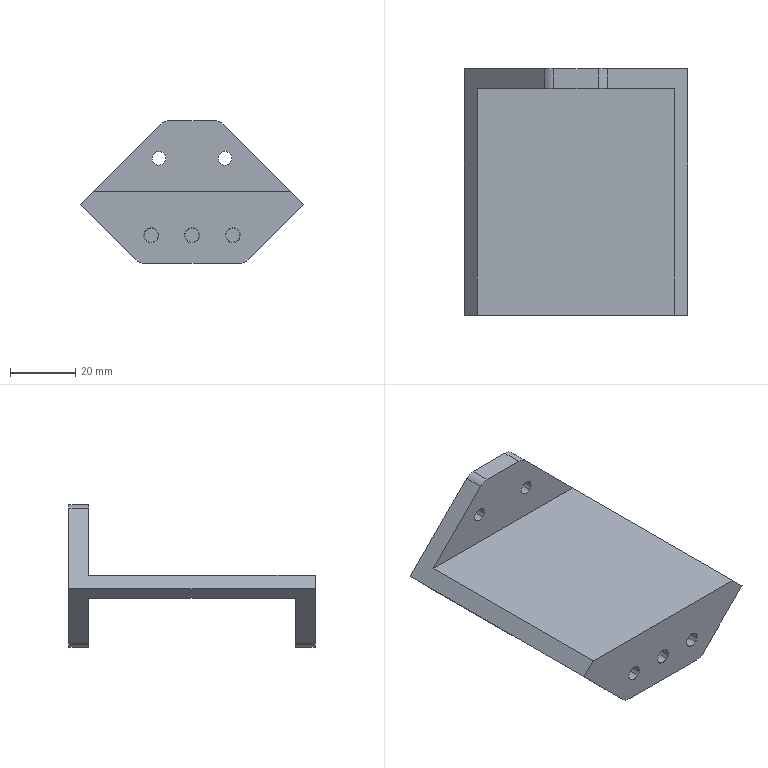NC program | NX | posted with a generic post | part box 68.307 x 75.3 x 43.668 mm
Lines 19 to 906 of 9000:
(ADAPTIVE_MILLING , TOOL : D10)
N36 T15 M6
N38 G54
N40 G17 G0 G90 X-31.665 Y-45.86 B0. C0. S9500 M3
N42 G43 Z30. H15
N44 Z-11.85
N46 G94 G1 Z-14.85 F1000.
N48 X-31.386 Y-45.079 F3000.
N50 X-31.129 Y-44.291
N52 G3 X-31.665 Y-43.213 R1.017
N54 X-34.729 Y-42.452 R8.28
N56 X-39.219 Y-42.188 R149.722
N58 G2 X-43.375 Y-39.245 R6.16
N60 X-45.215 Y-33.584 R13.81
N62 X-45.618 Y-24.224 R80.865
N64 G1 X-45.625 Y-22.724
N66 X-45.631 Y-20.599
N68 X-45.634 Y-17.349
N70 X-45.636 Y-9.599
N72 Y35.151
N74 X-45.629 Y35.401
N76 G2 X-43.02 Y39.625 R5.889
N78 X-37.31 Y41.673 R12.902
N80 X-28.577 Y42.113 R68.398
N82 G1 X-27.202 Y42.123
N84 X-25.702 Y42.13
N86 X-23.577 Y42.135
N88 X-19.952 Y42.138
N90 X-9.327 Y42.139
N92 X38.673
N94 G2 X42.915 Y39.817 R5.625
N96 X45.077 Y34.419 R11.908
N98 X45.604 Y25.819 R57.608
N100 G1 X45.614 Y24.694
N102 X45.621 Y23.444
N104 X45.628 Y21.694
N106 X45.633 Y19.319
N108 X45.635 Y14.944
N110 X45.636 Y-13.681
N112 Y-35.181
N114 X45.634 Y-35.306
N116 X45.627 Y-35.431
N118 X45.617 Y-35.555
N120 G2 X42.912 Y-39.721 R5.935
N122 X37.297 Y-41.68 R13.094
N124 X28.689 Y-42.113 R69.339
N126 G1 X27.439 Y-42.122
N128 X25.939 Y-42.129
N130 X23.814 Y-42.134
N132 X20.439 Y-42.138
N134 X11.689 Y-42.139
N136 X-27.811
N138 G2 X-33.408 Y-41.614 R60.129
N140 X-37.011 Y-41.244 R40.3
N142 X-42.457 Y-36.811 R8.328
N144 X-44.258 Y-30.091 R18.441
N146 X-44.608 Y-19.851 R114.492
N148 G1 X-44.615 Y-18.101
N150 X-44.621 Y-15.601
N152 X-44.624 Y-11.601
N154 X-44.625 Y-0.101
N156 Y32.149
N158 X-44.618 Y32.399
N160 G2 X-40.842 Y38.536 R7.705
N162 X-34.357 Y40.647 R15.817
N164 X-24.623 Y41.102 R84.301
N166 G1 X-23.373 Y41.111
N168 X-21.873 Y41.117
N170 X-19.623 Y41.123
N172 X-16.123 Y41.127
N174 X-7.873 Y41.128
N176 X35.502
N178 G2 X41.889 Y37.582 R7.573
N180 X44.088 Y31.26 R15.12
N182 X44.589 Y22.281 R70.625
N184 G1 X44.599 Y21.156
N186 X44.608 Y19.781
N188 X44.615 Y18.156
N190 X44.621 Y15.781
N192 X44.624 Y12.031
N194 X44.625 Y2.156
N196 Y-32.094
N198 X44.624 Y-32.219
N200 X44.615 Y-32.469
N202 X44.609 Y-32.594
N204 X44.6 Y-32.718
N206 G2 X40.792 Y-38.576 R7.743
N208 X34.544 Y-40.625 R15.694
N210 X25.187 Y-41.098 R77.266
N212 G1 X23.937 Y-41.108
N214 X22.312 Y-41.116
N216 X20.312 Y-41.122
N218 X17.187 Y-41.126
N220 X11.187 Y-41.128
N222 X-25.438
N224 G2 X-34.656 Y-40.436 R83.781
N226 X-41.245 Y-35.347 R9.432
N228 G1 X-41.361 Y-35.125
N230 X-41.417 Y-35.013
N232 X-41.472 Y-34.901
N234 X-41.525 Y-34.788
N236 X-41.578 Y-34.675
N238 X-41.63 Y-34.561
N240 X-41.73 Y-34.332
N242 X-41.779 Y-34.217
N244 X-41.827 Y-34.101
N246 X-41.873 Y-33.985
N248 X-41.923 Y-33.871
N250 X-41.974 Y-33.78
N252 G2 X-42.882 Y-31.037 R6.648
N254 X-43.558 Y-21.32 R65.424
N256 G1 X-43.571 Y-20.445
N258 X-43.583 Y-19.321
N260 X-43.592 Y-18.071
N262 X-43.6 Y-16.446
N264 X-43.607 Y-14.321
N266 X-43.611 Y-11.321
N268 X-43.614 Y-5.946
N270 X-43.615 Y29.304
N272 X-43.613 Y29.554
N274 X-43.612 Y29.679
N276 X-43.609 Y29.804
N278 X-43.601 Y30.054
N280 X-43.595 Y30.179
N282 G2 X-38.917 Y37.549 R8.918
N284 X-31.774 Y39.66 R18.511
N286 X-20.663 Y40.098 R106.491
N288 G1 X-18.913 Y40.106
N290 X-16.663 Y40.111
N292 X-13.288 Y40.115
N294 X-6.288 Y40.117
N296 X32.962 Y40.118
N298 X33.212 Y40.115
N300 G2 X41.065 Y35.398 R8.902
N302 G1 X41.128 Y35.29
N304 X41.189 Y35.181
N306 X41.307 Y34.96
N308 X41.364 Y34.849
N310 X41.42 Y34.738
N312 X41.53 Y34.513
N314 X41.583 Y34.4
N316 X41.688 Y34.173
N318 X41.723 Y34.111
N320 G2 X42.741 Y31.774 R5.072
N322 X43.532 Y22.569 R54.427
N324 X43.614 Y1.695 R975.422
N326 G1 X43.615 Y-29.43
N328 X43.612 Y-29.68
N330 X43.606 Y-29.93
N332 X43.602 Y-30.055
N334 X43.589 Y-30.305
N336 G2 X38.924 Y-37.552 R8.898
N338 X32.277 Y-39.599 R17.939
N340 X21.795 Y-40.089 R90.439
N342 G1 X20.42 Y-40.099
N344 X18.67 Y-40.106
N346 X16.295 Y-40.112
N348 X12.67 Y-40.116
N350 X4.42 Y-40.117
N352 X-23.705 Y-40.118
N354 G2 X-32.804 Y-39.541 R64.009
N356 X-38.655 Y-36.183 R10.283
N358 G3 X-40.291 Y-35.45 R29.243
N360 G2 X-42.026 Y-33.711 R5.781
N362 G1 X-42.148 Y-33.521
N364 X-42.605 Y-32.397
N366 X-42.64 Y-32.264
N368 X-42.796 Y-31.024
N370 X-42.8 Y-30.958
N372 Y30.958
N374 X-42.796 Y31.024
N376 G2 X-41.347 Y34.608 R5.58
N378 X-37.507 Y36.891 R13.071
N380 X-28.873 Y38.771 R27.669
N382 X-15.38 Y39.097 R191.104
N384 G1 X-12.505 Y39.103
N386 X-8.005 Y39.106
N388 X6.37 Y39.107
N390 X30.62
N392 X30.995 Y39.103
N394 X31.245 Y39.098
N396 G2 X38.235 Y36.245 R9.765
N398 G3 X39.054 Y35.991 R2.422
N400 G2 X41.347 Y34.608 R5.838
N402 G1 X41.724 Y34.11
N404 G3 X43.518 Y34.789 R1.001
N406 G1 X43.448 Y35.087 Z-14.835
N408 X43.331 Y35.371 Z-14.819
N410 X42.801 Y36.651 Z-14.75
N412 X42.476 Y37.441
N414 X42.137 Y38.226
N416 G3 X41.724 Y38.61 R1.054
N418 G1 X37.807 Y40.557
N420 G3 X34.63 Y41.648 R15.261
N422 X32.101 Y41.977 R26.338
N424 G1 X30.702 Y42.068
N426 X29.301 Y42.103
N428 X-18.201 Y42.154
N430 G3 X-28.49 Y41.809 R149.233
N432 X-35.16 Y40.765 R46.348
N434 G1 X-39.008 Y39.867
N436 G3 X-39.589 Y39.481 R1.032
N438 G1 X-40.629 Y38.048
N440 X-41.045 Y37.481 Z-14.785
N442 X-41.447 Y36.904 Z-14.82
N444 G3 X-41.554 Y36.33 Z-14.85 R1.049
N446 X-40.172 Y35.52 R1.003
N448 G2 X-37.932 Y36.172 R5.778
N450 X-28.564 Y37.701 R71.762
N452 X-13.947 Y38.085 R197.198
N454 G1 X-11.697 Y38.09
N456 X-7.947 Y38.094
N458 X-0.322 Y38.096
N460 X28.553
N462 X28.927 Y38.092
N464 X29.427 Y38.082
N466 G2 X35.518 Y36.429 R13.144
N468 G3 X36.153 Y36.203 R3.775
N470 G2 X38.677 Y36.061 R11.846
N472 G3 X38.828 Y38.251 R-1.1
N474 G1 X31.219 Y38.258
N476 X29.219 Y38.26 Z-14.75
N478 X-29.334 Y38.312
N480 X-31.334 Y38.314 Z-14.85
N482 X-38.327 Y38.32
N484 G3 X-38.178 Y36.13 R-1.1
N486 G1 X-37.686 Y36.198
N488 X-37.614 Y36.203
N490 G3 X-30.501 Y36.53 R56.138
N492 G2 X-13.515 Y37.07 R208.339
N494 G1 X-11.14 Y37.077
N496 X-7.89 Y37.081
N498 X-2.39 Y37.084
N500 X19.11 Y37.085
N502 X26.485
N504 X26.985 Y37.083
N506 G2 X32.731 Y36.203 R19.314
N508 G1 X36.231
N510 G3 X37.329 Y37.305 R1.1
N512 X36.231 Y38.403 R1.1
N514 G1 X31.619
N516 X29.619 Z-14.75
N518 X-29.592
N520 X-31.592 Z-14.85
N522 X-34.989
N524 G3 X-36.087 Y37.301 R1.1
N526 X-34.989 Y36.203 R1.1
N528 G1 X-31.686
N530 X-31.614 Y36.198
N532 G3 X-25.758 Y35.917 R31.279
N534 G2 X-1.884 Y36.073 R956.691
N536 G1 X12.116 Y36.075
N538 X24.616
N540 X25.366 Y36.07
N542 X25.741 Y36.063
N544 X25.991 Y36.057
N546 G2 X29.473 Y35.738 R41.584
N548 G3 X30.379 Y36.028 R4.567
N550 G2 X32.811 Y36.203 R10.972
N552 G3 X33.909 Y37.305 R1.1
N554 X32.808 Y38.403 R1.1
N556 G1 X31.571 Y38.399
N558 X29.571 Y38.392 Z-14.75
N560 X-29.041 Y38.192
N562 X-30.249 Y38.177 Z-14.81
N564 G3 X-30.926 Y37.801 Z-14.85 R1.132
N566 X-30.379 Y36.028 R1.102
N568 X-25.86 Y35.125 R12.1
N570 X-13.112 Y35.059 R322.419
N572 G1 X-12.237 Y35.061
N574 X-11.737 Y35.063
N576 X-10.487
N578 X-9.737 Y35.066
N580 X-8.737
N582 X-8.362
N584 X-7.362 Y35.069
N586 X-6.612
N588 X-5.612 Y35.071
N590 X-5.112 Y35.072
N592 X-4.362 Y35.071
N594 X-3.237 Y35.073
N596 X-2.862 Y35.074
N598 X-1.987 Y35.073
N600 X-0.737 Y35.075
N602 X0.513 Y35.072
N604 X1.138 Y35.074
N606 X2.638 Y35.073
N608 X3.513 Y35.071
N610 X4.138 Y35.073
N612 X5.513 Y35.072
N614 X6.138
N616 X7.263 Y35.075
N618 X8.263 Y35.073
N620 X9.513 Y35.076
N622 X10.138 Y35.075
N624 X11.638 Y35.076
N626 X12.138 Y35.077
N628 X13.138 Y35.074
N630 X14.513 Y35.077
N632 X15.638 Y35.074
N634 X16.388 Y35.075
N636 X17.263 Y35.074
N638 X17.763 Y35.073
N640 X18.638 Y35.075
N642 X19.888 Y35.073
N644 G2 X27.883 Y34.883 R129.556
N646 G3 X29.009 Y35.451 R1.838
N648 G1 X29.128 Y35.52
N650 X29.819 Y35.811
N652 G3 X30.291 Y37.458 R1.103
N654 X29.296 Y37.925 Z-14.793 R1.131
N656 G1 X28.445 Y37.924 Z-14.75
N658 X-28.234 Y37.863
N660 X-28.821 Y37.865 Z-14.779
N662 X-29.408 Y37.85 Z-14.809
N664 G3 X-30.105 Y37.445 Z-14.85 R1.13
N666 X-29.67 Y35.749 R1.103
N668 G2 X-28.24 Y35.038 R22.99
N670 G3 X-23.33 Y34.207 R16.333
N672 X-8.332 Y34.071 R360.005
N674 G1 X-7.832 Y34.072
N676 X-6.832 Y34.071
N678 X-5.707 Y34.073
N680 X-4.707 Y34.072
N682 X-3.707 Y34.074
N684 X-3.082
N686 X-2.332 Y34.073
N688 X-0.957 Y34.075
N690 X0.418 Y34.072
N692 X1.793 Y34.075
N694 X2.418 Y34.073
N696 X3.918 Y34.074
N698 X4.918 Y34.076
N700 X5.793 Y34.074
N702 X6.543 Y34.075
N704 X6.918 Y34.076
N706 X8.293 Y34.073
N708 G2 X23.793 Y34.017 R790.06
N710 G3 X27.283 Y34.08 R15.903
N712 X28.051 Y34.706 R1.755
N714 G1 X28.544 Y35.09
N716 G3 X28.832 Y36.49 R1.106
N718 X27.784 Y37.059 Z-14.787 R1.123
N720 G1 X27.042 Y37.064 Z-14.75
N722 X-27.468 Y37.414
N724 X-28.489 Y37.408 Z-14.801
N726 G3 X-29.277 Y36.885 Z-14.85 R1.117
N728 X-29.009 Y35.451 R1.106
N730 X-25.203 Y33.695 R7.328
N732 X-17.983 Y33.139 R44.306
N734 G1 X-17.108 Y33.125
N736 X-15.983 Y33.111
N738 X-14.733 Y33.1
N740 X-13.483 Y33.093
N742 X-12.733 Y33.09
N744 X-11.983 Y33.084
N746 X-11.108 Y33.081
N748 X17.392 Y33.082
N750 X17.892 Y33.079
N752 X20.391 Y33.061
N754 G3 X25.639 Y33.067 R60.63
N756 X27.062 Y33.478 R2.885
N758 G1 X27.155 Y33.562
N760 X27.221 Y33.641
N762 X27.825 Y34.438
N764 G3 X27.878 Y35.689 R1.108
N766 X26.78 Y36.204 Z-14.786 R1.183
N768 G1 X26.057 Y36.212 Z-14.75
N770 X-26.656 Y36.796
N772 X-27.692 Z-14.802
N774 G3 X-28.476 Y36.29 Z-14.85 R1.117
N776 X-28.219 Y34.837 R1.106
N778 X-27.214 Y33.943 R12.106
N780 X-22.949 Y32.611 R11.114
N782 X-14.343 Y32.133 R70.206
N784 G1 X-13.343 Y32.12
N786 X-12.343 Y32.111
N788 X-11.093 Y32.104
N790 X-9.218 Y32.098
N792 X-6.343 Y32.094
N794 X-0.593 Y32.092
N796 X14.407
N798 X14.907 Y32.09
N800 G3 X24.031 Y32.072 R239.487
N802 X26.574 Y32.634 R6.287
N804 X27.152 Y33.521 R1.675
N806 G1 X27.221 Y33.641
N808 X27.296 Y33.741
N810 G3 X27.352 Y34.989 R1.108
N812 X26.255 Y35.507 Z-14.786 R1.183
N814 G1 X25.532 Y35.518 Z-14.75
N816 X-26.08 Y36.26
N818 X-26.624 Y36.271 Z-14.777
N820 X-27.167 Y36.26 Z-14.804
N822 G3 X-27.915 Y35.785 Z-14.85 R1.127
N824 X-27.878 Y34.508 R1.108
N826 X-25. Y32.426 R5.204
N828 X-18.61 Y31.349 R24.488
N830 X-4.614 Y31.107 R256.473
N832 G1 X-0.489 Y31.104
N834 X11.386 Y31.103
N836 X11.886 Y31.1
N838 G3 X22.635 Y31.084 R342.387
N840 X26.16 Y31.801 R8.623
N842 X26.695 Y32.397 R1.269
N844 G1 X26.978 Y33.092
N846 G3 X26.808 Y34.206 R1.112
N848 X25.79 Y34.61 Z-14.793 R1.215
N850 G1 X24.93 Y34.628 Z-14.75
N852 X-25.608 Y35.656
N854 X-26.157 Y35.671 Z-14.777
N856 X-26.706 Y35.664 Z-14.805
N858 G3 X-27.452 Y35.203 Z-14.85 R1.127
N860 X-27.425 Y33.911 R1.108
N862 X-24.67 Y31.711 R5.118
N864 X-18.317 Y30.449 R22.393
N866 X-4.824 Y30.123 R190.213
N868 G1 X-2.074 Y30.118
N870 X2.301 Y30.115
N872 X8.426 Y30.114
N874 X8.926 Y30.111
N876 X10.426 Y30.101
N878 X11.051 Y30.1
N880 X12.176 Y30.093
N882 G3 X22.049 Y30.129 R195.88
N884 X25.694 Y30.906 R9.913
N886 X26.66 Y32.264 R1.466
N888 G1 X26.691 Y32.385
N890 G3 X26.467 Y33.373 R1.116
N892 X25.46 Y33.767 Z-14.794 R1.223
N894 G1 X24.583 Y33.789 Z-14.75
N896 X-25.125 Y35.011
N898 X-25.7 Y35.028 Z-14.779
N900 X-26.276 Y35.027 Z-14.808
N902 G3 X-26.996 Y34.618 Z-14.85 R1.129
N904 X-27.152 Y33.521 R1.112
N906 X-25.276 Y31.434 R3.812
N908 X-19.931 Y29.788 R15.223
N910 X-9.831 Y29.184 R79.227
N912 G1 X-8.831 Y29.171
N914 X-7.581 Y29.158
N916 X-6.081 Y29.148
N918 X-4.331 Y29.139
N920 X-2.081 Y29.133
N922 X1.044 Y29.128
N924 X5.544 Y29.125
N926 X7.419 Y29.112
N928 X8.169 Y29.111
N930 X9.294 Y29.105
N932 X10.418 Y29.097
N934 X11.418 Y29.095
N936 G3 X21.291 Y29.164 R170.676
N938 X25.528 Y30.126 R10.894
N940 X26.524 Y31.183 R1.743
N942 G1 X26.618 Y31.927
N944 G3 X26.277 Y32.867 R1.116
N946 X25.371 Y33.169 Z-14.801 R1.236
N948 G1 X24.354 Y33.196 Z-14.75
N950 X-24.875 Y34.544
N952 X-25.475 Y34.562 Z-14.78
N954 X-26.075 Y34.565 Z-14.81
N956 G3 X-26.768 Y34.203 Z-14.85 R1.132
N958 X-26.964 Y33.058 R1.111
N960 X-24.796 Y30.583 R4.334
N962 X-19.092 Y28.832 R16.394
N964 X-8.994 Y28.207 R80.514
N966 G1 X-7.994 Y28.192
N968 X-6.869 Y28.178
N970 X-5.494 Y28.166
N972 X-3.869 Y28.156
N974 X-1.994 Y28.148
N976 X0.631 Y28.142
N978 X2.506 Y28.139
N980 X3.506 Y28.132
N982 X4.256 Y28.13
N984 X5.381 Y28.122
N986 X6.381 Y28.12
N988 X7.631 Y28.111
N990 X8.631 Y28.108
N992 X9.256 Y28.104
N994 X10.006 Y28.098
N996 X10.756 Y28.096
N998 G3 X20.504 Y28.191 R154.869
N1000 X25.23 Y29.251 R12.567
N1002 X26.425 Y30.304 R2.404
N1004 X26.535 Y31.272 R5.757
N1006 X26.133 Y32.266 R1.112
N1008 X25.278 Y32.514 Z-14.805 R1.281
N1010 G1 X24.189 Y32.546 Z-14.75
N1012 X-24.629 Y33.963
N1014 X-25.836 Y33.987 Z-14.81
N1016 G3 X-26.526 Y33.631 Z-14.85 R1.132
N1018 X-26.728 Y32.479 R1.111
N1020 X-25.119 Y30.213 R3.683
N1022 X-19.924 Y28.163 R13.518
N1024 X-10.852 Y27.296 R54.918
N1026 X10.647 Y27.095 R999.171
N1028 X20.018 Y27.235 R135.2
N1030 X25.095 Y28.432 R13.579
N1032 X26.402 Y29.556 R3.006
N1034 X26.5 Y30.673 R2.968
N1036 X26.051 Y31.56 R1.116
N1038 X25.246 Y31.779 Z-14.808 R1.29
N1040 G1 X24.097 Y31.818 Z-14.75
N1042 X-24.421 Y33.462
N1044 X-25.064 Y33.489 Z-14.782
N1046 X-25.709 Y33.492 Z-14.815
N1048 G3 X-26.337 Y33.187 Z-14.85 R1.143
N1050 X-26.66 Y32.264 R1.116
N1052 X-25.246 Y29.724 R3.468
N1054 X-20.29 Y27.446 R12.353
N1056 X-11.369 Y26.373 R45.968
N1058 X11.253 Y26.107 R715.221
N1060 X20.245 Y26.349 R87.619
N1062 X25.152 Y27.703 R12.778
N1064 X26.419 Y28.871 R2.969
N1066 X26.5 Y29.952 R3.319
N1068 X25.986 Y30.883 R1.113
N1070 X25.252 Y31.059 Z-14.812 R1.327
N1072 G1 X24.019 Y31.106 Z-14.75
N1074 X-24.253 Y32.957
N1076 X-24.937 Y32.986 Z-14.784
N1078 X-25.621 Y32.999 Z-14.819
N1080 G3 X-26.196 Y32.761 Z-14.85 R1.153
N1082 X-26.598 Y31.768 R1.112
N1084 X-25.111 Y28.992 R3.753
N1086 X-19.955 Y26.559 R12.83
N1088 X-10.918 Y25.414 R45.657
N1090 X16.578 Y25.166 R596.971
N1092 X23.245 Y26.086 R25.616
N1094 X26.24 Y27.815 R6.59
N1096 X26.5 Y28.443 R1.55
N1098 G1 Y29.318
N1100 G3 X25.979 Y30.254 R1.113
N1102 X25.252 Y30.425 Z-14.812 R1.335
N1104 G1 X24.01 Y30.473 Z-14.75
N1106 X-24.152 Y32.336
N1108 X-25.539 Y32.379 Z-14.819
N1110 G3 X-26.1 Y32.155 Z-14.85 R1.156
N1112 X-26.52 Y31.147 R1.112
N1114 X-25.327 Y28.555 R3.487
N1116 X-20.433 Y25.893 R11.764
N1118 X-11.685 Y24.523 R38.906
N1120 X6.559 Y24.132 R367.265
N1122 X17.806 Y24.286 R168.743
N1124 X24.025 Y25.553 R19.875
N1126 X26.345 Y27.19 R5.403
N1128 G1 X26.5 Y27.668
N1130 Y28.543
N1132 G3 X25.978 Y29.479 R1.113
N1134 X25.255 Y29.65 Z-14.812 R1.339
N1136 G1 X24.01 Y29.703 Z-14.75
N1138 X-24.071 Y31.752
N1140 X-24.801 Y31.789 Z-14.787
N1142 X-25.532 Y31.8 Z-14.823
N1144 X-25.791 Y31.732 Z-14.837
N1146 X-26.029 Y31.61 Z-14.85
N1148 G3 X-26.5 Y30.708 R1.116
N1150 X-25.43 Y28.003 R3.502
N1152 X-20.761 Y25.202 R11.243
N1154 X-12.051 Y23.624 R35.558
N1156 X3.065 Y23.174 R247.766
N1158 X16.562 Y23.269 R235.069
N1160 X23.43 Y24.483 R23.969
N1162 X26.256 Y26.262 R6.78
N1164 X26.5 Y26.867 R1.695
N1166 G1 Y27.742
N1168 G3 X25.978 Y28.678 R1.112
N1170 X25.261 Y28.85 Z-14.813 R1.345
N1172 G1 X24.01 Y28.911 Z-14.75
N1174 X-24.009 Y31.241
N1176 X-24.76 Y31.282 Z-14.788
N1178 X-25.512 Y31.302 Z-14.825
N1180 X-25.752 Y31.246 Z-14.838
N1182 X-25.977 Y31.144 Z-14.85
N1184 G3 X-26.5 Y30.208 R1.112
N1186 X-25.385 Y27.262 R3.757
N1188 X-20.635 Y24.354 R11.638
N1190 X-11.567 Y22.664 R36.07
N1192 X5.173 Y22.173 R256.984
N1194 X16.669 Y22.335 R158.056
N1196 X23.628 Y23.723 R23.026
N1198 X26.299 Y25.512 R6.447
N1200 X26.5 Y26.068 R2.148
N1202 G1 Y26.943
N1204 G3 X25.978 Y27.879 R1.112
N1206 X25.264 Y28.052 Z-14.813 R1.349
N1208 G1 X24.01 Y28.117 Z-14.75
N1210 X-23.994 Y30.611
N1212 X-24.749 Y30.654 Z-14.788
N1214 X-25.505 Y30.678 Z-14.826
N1216 X-25.742 Y30.624 Z-14.838
N1218 X-25.964 Y30.527 Z-14.85
N1220 G3 X-26.5 Y29.583 R1.112
N1222 X-25.273 Y26.425 R3.967
N1224 X-20.291 Y23.419 R12.343
N1226 X-10.975 Y21.691 R37.38
N1228 X5.889 Y21.184 R248.054
N1230 X17.255 Y21.454 R113.525
N1232 X24.036 Y23.055 R21.152
N1234 X26.329 Y24.741 R5.988
N1236 X26.5 Y25.244 R4.161
N1238 G1 Y26.119
N1240 G3 X25.977 Y27.055 R1.112
N1242 X25.268 Y27.228 Z-14.813 R1.367
N1244 G1 X24.01 Y27.298 Z-14.75
N1246 X-23.994 Y29.981
N1248 X-24.747 Y30.027 Z-14.788
N1250 X-25.502 Y30.053 Z-14.826
N1252 X-25.74 Y30. Z-14.838
N1254 X-25.964 Y29.902 Z-14.85
N1256 G3 X-26.5 Y28.958 R1.112
N1258 X-25.256 Y25.676 R4.111
N1260 X-20.311 Y22.607 R12.506
N1262 X-11.392 Y20.802 R35.936
N1264 X3.968 Y20.219 R197.271
N1266 X15.838 Y20.397 R147.671
N1268 X23.405 Y21.927 R25.574
N1270 X26.286 Y23.85 R7.054
N1272 X26.5 Y24.429 R1.888
N1274 G1 Y25.304
N1276 G3 X25.977 Y26.241 R1.112
N1278 X25.269 Y26.414 Z-14.813 R1.369
N1280 G1 X24.01 Y26.486 Z-14.75
N1282 X-23.994 Y29.229
N1284 X-24.747 Y29.276 Z-14.788
N1286 X-25.501 Y29.303 Z-14.826
N1288 X-25.74 Y29.25 Z-14.838
N1290 X-25.964 Y29.152 Z-14.85
N1292 G3 X-26.5 Y28.208 R1.112
N1294 X-25.252 Y24.923 R4.193
N1296 X-20.226 Y21.751 R12.717
N1298 X-11.322 Y19.874 R35.586
N1300 X4.16 Y19.237 R182.936
N1302 X16.152 Y19.488 R120.826
N1304 X23.45 Y21.087 R24.765
N1306 X26.308 Y23.042 R6.971
N1308 X26.5 Y23.581 R2.45
N1310 G1 Y24.456
N1312 G3 X25.977 Y25.393 R1.112
N1314 X25.271 Y25.566 Z-14.813 R1.372
N1316 G1 X24.01 Y25.64 Z-14.75
N1318 X-23.994 Y28.476
N1320 X-24.746 Y28.525 Z-14.788
N1322 X-25.499 Y28.553 Z-14.825
N1324 X-25.739 Y28.5 Z-14.838
N1326 X-25.964 Y28.402 Z-14.85
N1328 G3 X-26.5 Y27.458 R1.112
N1330 X-25.258 Y24.168 R4.254
N1332 X-20.153 Y20.889 R12.966
N1334 X-10.89 Y18.906 R36.206
N1336 X5.466 Y18.243 R188.956
N1338 X17.199 Y18.673 R89.943
N1340 X24.164 Y20.557 R21.586
N1342 X26.386 Y22.329 R5.518
N1344 X26.5 Y23.605 R3.126
N1346 X25.977 Y24.541 R1.112
N1348 X25.275 Y24.715 Z-14.813 R1.377
N1350 G1 X24.01 Y24.795 Z-14.75
N1352 X-23.994 Y27.845
N1354 X-24.744 Y27.898 Z-14.788
N1356 X-25.495 Y27.928 Z-14.825
N1358 X-25.737 Y27.876 Z-14.838
N1360 X-25.963 Y27.777 Z-14.85
N1362 G3 X-26.5 Y26.833 R1.112
N1364 X-25.271 Y23.41 R4.371
N1366 X-20.203 Y20.072 R13.063
N1368 X-10.715 Y17.962 R36.054
N1370 X4.639 Y17.272 R172.068
N1372 X16.499 Y17.663 R95.948
N1374 X23.742 Y19.484 R23.837
N1376 X26.337 Y21.386 R6.695
N1378 X26.5 Y21.875 R6.215
N1380 G1 Y22.75
N1382 G3 X25.977 Y23.687 R1.112
N1384 X25.277 Y23.86 Z-14.814 R1.38
N1386 G1 X24.01 Y23.943 Z-14.75
N1388 X-23.994 Y27.093
N1390 X-24.743 Y27.146 Z-14.788
N1392 X-25.494 Y27.179 Z-14.825
N1394 X-25.736 Y27.126 Z-14.838
N1396 X-25.963 Y27.028 Z-14.85
N1398 G3 X-26.5 Y26.083 R1.112
N1400 X-25.21 Y22.555 R4.477
N1402 X-20.03 Y19.159 R13.513
N1404 X-10.548 Y17.018 R36.446
N1406 X5.554 Y16.283 R170.558
N1408 X17.156 Y16.822 R81.323
N1410 X24.209 Y18.85 R21.831
N1412 X26.345 Y20.543 R6.042
N1414 G1 X26.5 Y21.021
N1416 Y21.896
N1418 G3 X25.977 Y22.833 R1.112
N1420 X25.277 Y23.007 Z-14.814 R1.379
N1422 G1 X24.01 Y23.089 Z-14.75
N1424 X-23.994 Y26.218
N1426 X-24.743 Y26.272 Z-14.788
N1428 X-25.494 Y26.304 Z-14.825
N1430 X-25.736 Y26.251 Z-14.838
N1432 X-25.963 Y26.153 Z-14.85
N1434 G3 X-26.5 Y25.208 R1.112
N1436 X-25.238 Y21.792 R4.467
N1438 X-19.982 Y18.29 R13.628
N1440 X-10.389 Y16.074 R37.186
N1442 X6.086 Y15.304 R164.27
N1444 X17.802 Y15.998 R72.241
N1446 X24.441 Y18.104 R20.35
N1448 X26.406 Y19.797 R4.974
N1450 X26.5 Y21.034 R3.473
N1452 X25.977 Y21.971 R1.112
N1454 X25.279 Y22.145 Z-14.814 R1.382
N1456 G1 X24.01 Y22.23 Z-14.75
N1458 X-23.994 Y25.465
N1460 X-24.742 Y25.52 Z-14.788
N1462 X-25.492 Y25.554 Z-14.825
N1464 X-25.735 Y25.502 Z-14.838
N1466 X-25.963 Y25.403 Z-14.85
N1468 G3 X-26.5 Y24.458 R1.112
N1470 X-25.272 Y21.028 R4.508
N1472 X-20.169 Y17.518 R13.488
N1474 X-10.608 Y15.177 R35.818
N1476 X5.237 Y14.335 R147.991
N1478 X17.083 Y14.964 R77.315
N1480 X24.012 Y16.991 R22.893
N1482 X26.354 Y18.818 R6.322
N1484 G1 X26.5 Y19.293
N1486 Y20.168
N1488 G3 X25.976 Y21.105 R1.112
N1490 X25.281 Y21.279 Z-14.814 R1.386
N1492 G1 X24.01 Y21.368 Z-14.75
N1494 X-23.994 Y24.712
N1496 X-24.741 Y24.769 Z-14.788
N1498 X-25.49 Y24.804 Z-14.825
N1500 X-25.734 Y24.752 Z-14.838
N1502 X-25.963 Y24.653 Z-14.85
N1504 G3 X-26.5 Y23.708 R1.112
N1506 X-25.233 Y20.164 R4.633
N1508 X-19.903 Y16.547 R14.025
N1510 X-10.214 Y14.201 R37.121
N1512 X12.876 Y13.567 R142.698
N1514 X22.185 Y15.307 R35.071
N1516 X26.046 Y17.549 R10.363
N1518 X26.5 Y18.413 R1.461
N1520 G1 Y19.413
N1522 G3 X25.977 Y20.35 R1.112
N1524 X25.281 Y20.524 Z-14.814 R1.386
N1526 G1 X24.01 Y20.613 Z-14.75
N1528 X-23.994 Y23.962
N1530 X-24.741 Y24.019 Z-14.788
N1532 X-25.49 Y24.054 Z-14.825
N1534 X-25.734 Y24.002 Z-14.838
N1536 X-25.963 Y23.903 Z-14.85
N1538 G3 X-26.5 Y22.958 R1.112
N1540 X-25.198 Y19.301 R4.72
N1542 X-19.874 Y15.671 R14.256
N1544 X-9.701 Y13.209 R37.987
N1546 X12.764 Y12.613 R133.908
N1548 X22.188 Y14.414 R35.104
N1550 X26.044 Y16.664 R10.44
N1552 X26.5 Y17.53 R1.475
N1554 G1 Y18.53
N1556 G3 X25.977 Y19.467 R1.112
N1558 X25.281 Y19.641 Z-14.814 R1.386
N1560 G1 X24.01 Y19.73 Z-14.75
N1562 X-23.994 Y23.087
N1564 X-24.741 Y23.144 Z-14.788
N1566 X-25.49 Y23.179 Z-14.825
N1568 X-25.734 Y23.127 Z-14.838
N1570 X-25.963 Y23.028 Z-14.85
N1572 G3 X-26.5 Y22.083 R1.112
N1574 X-25.248 Y18.531 R4.689
N1576 X-19.849 Y14.793 R14.414
N1578 X-9.813 Y12.293 R37.952
N1580 X13.021 Y11.691 R124.856
N1582 X22.422 Y13.605 R34.482
N1584 X26.122 Y15.869 R9.805
N1586 X26.5 Y16.64 R1.426
N1588 G1 Y17.64
N1590 G3 X25.976 Y18.577 R1.112
N1592 X25.284 Y18.752 Z-14.814 R1.39
N1594 G1 X24.01 Y18.844 Z-14.75
N1596 X-23.994 Y22.333
N1598 X-24.74 Y22.392 Z-14.787
N1600 X-25.488 Y22.429 Z-14.825
N1602 X-25.733 Y22.377 Z-14.837
N1604 X-25.962 Y22.278 Z-14.85
N1606 G3 X-26.5 Y21.333 R1.112
N1608 X-25.219 Y17.664 R4.806
N1610 X-19.828 Y13.914 R14.53
N1612 X-9.308 Y11.302 R38.9
N1614 X13.15 Y10.758 R118.456
N1616 X22.301 Y12.658 R34.462
N1618 X26.033 Y14.879 R10.513
N1620 X26.5 Y15.751 R1.546
N1622 G1 Y16.751
N1624 G3 X25.976 Y17.688 R1.112
N1626 X25.284 Y17.863 Z-14.814 R1.39
N1628 G1 X24.01 Y17.956 Z-14.75
N1630 X-23.994 Y21.458
N1632 X-24.74 Y21.517 Z-14.787
N1634 X-25.487 Y21.554 Z-14.825
N1636 X-25.732 Y21.502 Z-14.837
N1638 X-25.962 Y21.403 Z-14.85
N1640 G3 X-26.5 Y20.458 R1.112
N1642 X-25.276 Y16.893 R4.758
N1644 X-20.154 Y13.189 R14.143
N1646 X-10.42 Y10.527 R36.315
N1648 X13.398 Y9.839 R111.334
N1650 X22.525 Y11.844 R33.555
N1652 X26.105 Y14.071 R9.842
N1654 X26.5 Y14.859 R1.436
N1656 G1 Y15.859
N1658 G3 X25.976 Y16.795 R1.112
N1660 X25.284 Y16.97 Z-14.814 R1.39
N1662 G1 X24.011 Y17.063 Z-14.75
N1664 X-23.994 Y20.582
N1666 X-24.74 Y20.642 Z-14.787
N1668 X-25.487 Y20.679 Z-14.825
N1670 X-25.732 Y20.627 Z-14.837
N1672 X-25.962 Y20.528 Z-14.85
N1674 G3 X-26.5 Y19.583 R1.112
N1676 X-25.259 Y16.023 R4.774
N1678 X-19.801 Y12.155 R14.637
N1680 X-9.556 Y9.47 R38.604
N1682 X12.894 Y8.855 R107.354
N1684 X22.281 Y10.841 R35.4
N1686 X26.092 Y13.166 R10.38
N1688 X26.5 Y13.969 R1.466
N1690 G1 Y14.969
N1692 G3 X25.976 Y15.906 R1.112
N1694 X25.287 Y16.081 Z-14.814 R1.394
N1696 G1 X24.011 Y16.178 Z-14.75
N1698 X-23.994 Y19.829
N1700 X-24.739 Y19.89 Z-14.787
N1702 X-25.485 Y19.929 Z-14.825
N1704 X-25.731 Y19.878 Z-14.837
N1706 X-25.962 Y19.778 Z-14.85
N1708 G3 X-26.5 Y18.833 R1.112
N1710 X-25.243 Y15.152 R4.882
N1712 X-19.906 Y11.323 R14.727
N1714 X-9.806 Y8.576 R38.056
N1716 X13.633 Y7.991 R100.911
N1718 X22.731 Y10.119 R32.842
N1720 X26.162 Y12.35 R9.6
N1722 X26.5 Y13.075 R1.443
N1724 G1 Y14.075
N1726 G3 X25.976 Y15.012 R1.112
N1728 X25.287 Y15.186 Z-14.814 R1.395
N1730 G1 X24.011 Y15.284 Z-14.75
N1732 X-23.994 Y18.953
N1734 X-24.738 Y19.015 Z-14.787
N1736 X-25.484 Y19.054 Z-14.825
N1738 X-25.731 Y19.003 Z-14.837
N1740 X-25.962 Y18.903 Z-14.85
N1742 G3 X-26.5 Y17.958 R1.112
N1744 X-25.229 Y14.281 R4.907
N1746 X-19.9 Y10.439 R14.849
N1748 X-9.813 Y7.645 R38.337
N1750 X13.374 Y7.025 R97.872
N1752 X22.483 Y9.109 R34.132
N1754 X26.146 Y11.437 R9.944
N1756 X26.5 Y12.184 R1.415
N1758 G1 Y13.184
N1760 G3 X25.976 Y14.121 R1.112
N1762 X25.288 Y14.295 Z-14.814 R1.395
N1764 G1 X24.011 Y14.393 Z-14.75
N1766 X-23.994 Y18.078
N1768 X-24.738 Y18.14 Z-14.787
N1770 X-25.484 Y18.179 Z-14.825
N1772 X-25.731 Y18.128 Z-14.837
N1774 X-25.962 Y18.028 Z-14.85
N1776 G3 X-26.5 Y17.083 R1.112
N1778 X-25.297 Y13.507 R4.847
N1780 X-20.012 Y9.606 R14.699
N1782 X-9.948 Y6.736 R37.6
N1784 X13.234 Y6.07 R94.954
N1786 X22.578 Y8.241 R34.228
N1788 X26.21 Y10.613 R9.69
N1790 X26.5 Y11.292 R1.45
N1792 G1 Y12.292
N1794 G3 X25.976 Y13.229 R1.112
N1796 X25.288 Y13.404 Z-14.814 R1.396
N1798 G1 X24.011 Y13.502 Z-14.75
N1800 X-23.994 Y17.202
N1802 X-24.738 Y17.265 Z-14.787
N1804 X-25.484 Y17.304 Z-14.825